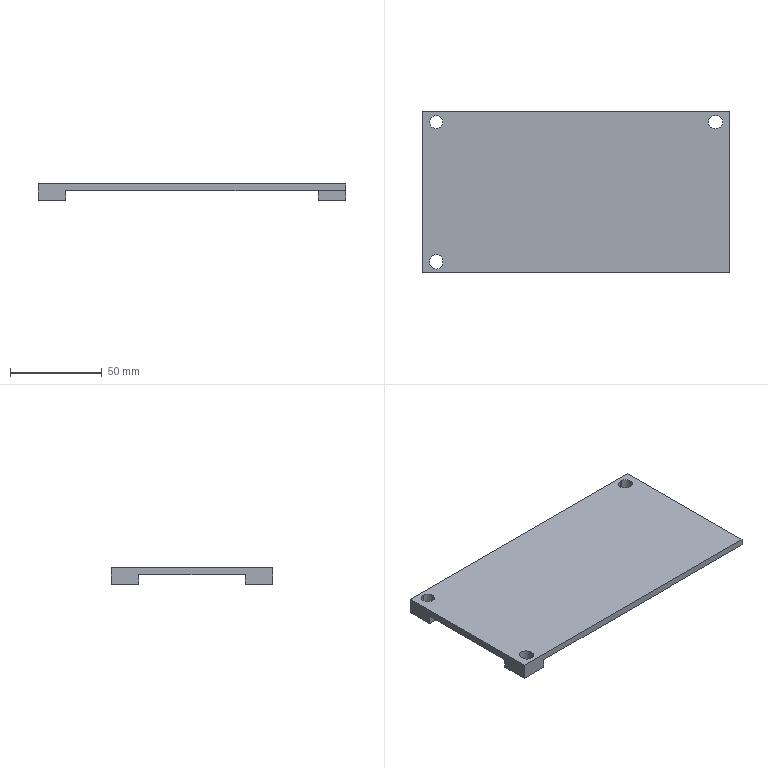NC program | NX | posted with a generic post | part box 168 x 88.2 x 8.8 mm
Lines 6927 to 6992 of 6992:
(PLANAR_PROFILE , TOOL : D6A45)
N13834 T01 M6
N13836 G54
N13838 G17 G0 G90 X77.849 Y39.247 S9500 M3
N13840 G43 Z30. H1
N13842 Z0.5
N13844 G94 G1 Z-1. F1500.
N13846 X77.135 Y40.485
N13848 G3 X76.615 Y40.785 R0.6
N13850 G1 X75.785
N13852 G3 X73.1 Y38.1 R2.685
N13854 X75.785 Y35.415 R2.685
N13856 G1 X76.615
N13858 G3 X79.3 Y38.1 R2.685
N13860 X76.615 Y40.785 R2.685
N13862 X76.095 Y40.485 R0.6
N13864 G1 X75.69 Y39.782
N13866 Z0.5
N13868 G0 Z30.
N13870 X-85.723 Y-44.822
N13872 Z0.5
N13874 G1 Z-1.
N13876 X-85.2 Y-44.52
N13878 G3 X-84.9 Y-44. R0.6
N13880 G1 Y44.
N13882 G2 X-83.9 Y45. R1.
N13884 G1 X83.9
N13886 G2 X84.9 Y44. R1.
N13888 G1 Y-44.
N13890 G2 X83.9 Y-45. R1.
N13892 G1 X-83.9
N13894 G2 X-84.9 Y-44. R1.
N13896 G3 X-85.2 Y-43.48 R0.6
N13898 G1 X-85.9 Y-43.076
N13900 Z0.5
N13902 G0 Z30.
N13904 X-74.966 Y39.247
N13906 Z0.5
N13908 G1 Z-1.
N13910 X-75.68 Y40.485
N13912 G3 X-76.2 Y40.785 R0.6
N13914 X-78.885 Y38.1 R2.685
N13916 X-76.2 Y40.785 R-2.685
N13918 X-76.72 Y40.485 R0.6
N13920 G1 X-77.434 Y39.247
N13922 Z0.5
N13924 G0 Z30.
N13926 X-77.347 Y-36.451
N13928 Z0.5
N13930 G1 Z-1.
N13932 X-78.585 Y-37.165
N13934 G3 X-78.885 Y-37.685 R0.6
N13936 G1 Y-38.515
N13938 G3 X-76.2 Y-41.2 R2.685
N13940 X-73.515 Y-38.515 R2.685
N13942 G1 Y-37.685
N13944 G3 X-76.2 Y-35. R2.685
N13946 X-78.885 Y-37.685 R2.685
N13948 X-78.585 Y-38.205 R0.6
N13950 G1 X-77.882 Y-38.61
N13952 Z0.5
N13954 G0 Z30.
N13956 M5
N13958 M2